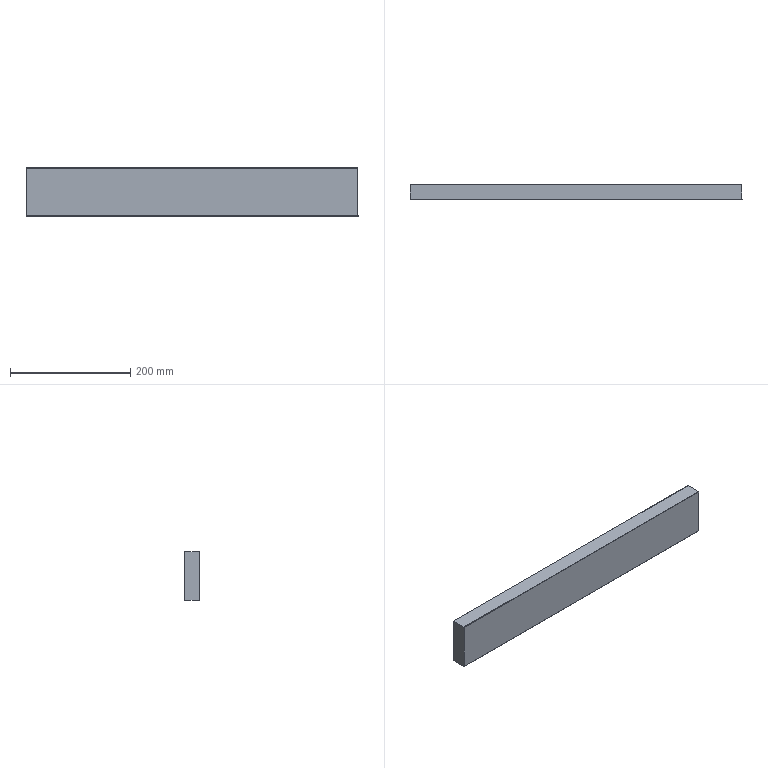Part | STEP file | DEWALT-DWE7492-B22 | 1 solid | 10 faces | box 552.2 x 25.6 x 80 mm | volume 1130787 mm3 | plane 6 | cylinder 4 | commonest cylinder face diameters 1 x4
STEP:
#1=CARTESIAN_POINT('',(0.,0.,0.));
#2=DIRECTION('',(0.,0.,1.));
#3=DIRECTION('',(1.,0.,0.));
#4=AXIS2_PLACEMENT_3D('',#1,#2,#3);
#5=CARTESIAN_POINT('',(-285.1,166.3,40.));
#6=VERTEX_POINT('',#5);
#7=CARTESIAN_POINT('',(-285.1,166.8,40.5));
#8=VERTEX_POINT('',#7);
#9=CARTESIAN_POINT('',(-285.1,166.3,40.5));
#10=DIRECTION('',(1.,0.,0.));
#11=DIRECTION('',(0.,0.,-1.));
#12=AXIS2_PLACEMENT_3D('',#9,#10,#11);
#13=CIRCLE('',#12,0.5);
#14=CARTESIAN_POINT('',(-285.1,166.3,40.5));
#15=DIRECTION('',(1.,0.,0.));
#16=DIRECTION('',(0.,0.,-1.));
#17=AXIS2_PLACEMENT_3D('',#14,#15,#16);
#18=CYLINDRICAL_SURFACE('',#17,0.5);
#19=CARTESIAN_POINT('',(0.,0.));
#20=DIRECTION('',(1.,0.));
#21=VECTOR('',#20,1.);
#22=LINE('',#19,#21);
#23=(GEOMETRIC_REPRESENTATION_CONTEXT(2)PARAMETRIC_REPRESENTATION_CONTEXT()REPRESENTATION_CONTEXT('',''));
#24=DEFINITIONAL_REPRESENTATION('',(#22),#23);
#25=PCURVE('',#18,#24);
#26=CARTESIAN_POINT('',(-285.1,141.19,39.99));
#27=DIRECTION('',(-1.,0.,0.));
#28=DIRECTION('',(0.,0.,1.));
#29=AXIS2_PLACEMENT_3D('',#26,#27,#28);
#30=PLANE('',#29);
#31=CARTESIAN_POINT('',(0.01,25.11));
#32=CARTESIAN_POINT('',(0.01,25.976));
#33=CARTESIAN_POINT('',(0.76,25.543));
#34=CARTESIAN_POINT('',(1.51,25.11));
#35=CARTESIAN_POINT('',(0.76,24.677));
#36=CARTESIAN_POINT('',(0.01,24.244));
#37=CARTESIAN_POINT('',(0.01,25.11));
#38=(BOUNDED_CURVE()B_SPLINE_CURVE(2,(#31,#32,#33,#34,#35,#36,#37),.UNSPECIFIED.,.T.,.F.)B_SPLINE_CURVE_WITH_KNOTS((1,2,2,2,2,1),(-2.094,0.,2.094,4.189,6.283,8.378),.UNSPECIFIED.)CURVE()GEOMETRIC_REPRESENTATION_ITEM()RATIONAL_B_SPLINE_CURVE((1.,0.5,1.,0.5,1.,0.5,1.))REPRESENTATION_ITEM(''));
#39=(GEOMETRIC_REPRESENTATION_CONTEXT(2)PARAMETRIC_REPRESENTATION_CONTEXT()REPRESENTATION_CONTEXT('',''));
#40=DEFINITIONAL_REPRESENTATION('',(#38),#39);
#41=PCURVE('',#30,#40);
#42=SURFACE_CURVE('',#13,(#25,#41),.PCURVE_S1.);
#43=EDGE_CURVE('',#6,#8,#42,.T.);
#44=ORIENTED_EDGE('',*,*,#43,.T.);
#45=CARTESIAN_POINT('',(267.1,166.8,40.5));
#46=VERTEX_POINT('',#45);
#47=CARTESIAN_POINT('',(-9.,166.8,40.5));
#48=DIRECTION('',(1.,0.,0.));
#49=VECTOR('',#48,1.);
#50=LINE('',#47,#49);
#51=CARTESIAN_POINT('',(1.571,276.1));
#52=DIRECTION('',(0.,1.));
#53=VECTOR('',#52,1.);
#54=LINE('',#51,#53);
#55=(GEOMETRIC_REPRESENTATION_CONTEXT(2)PARAMETRIC_REPRESENTATION_CONTEXT()REPRESENTATION_CONTEXT('',''));
#56=DEFINITIONAL_REPRESENTATION('',(#54),#55);
#57=PCURVE('',#18,#56);
#58=CARTESIAN_POINT('',(267.11,166.8,119.51));
#59=DIRECTION('',(0.,1.,0.));
#60=DIRECTION('',(0.,0.,-1.));
#61=AXIS2_PLACEMENT_3D('',#58,#59,#60);
#62=PLANE('',#61);
#63=CARTESIAN_POINT('',(79.01,276.11));
#64=DIRECTION('',(0.,-1.));
#65=VECTOR('',#64,1.);
#66=LINE('',#63,#65);
#67=(GEOMETRIC_REPRESENTATION_CONTEXT(2)PARAMETRIC_REPRESENTATION_CONTEXT()REPRESENTATION_CONTEXT('',''));
#68=DEFINITIONAL_REPRESENTATION('',(#66),#67);
#69=PCURVE('',#62,#68);
#70=SURFACE_CURVE('',#50,(#57,#69),.PCURVE_S1.);
#71=EDGE_CURVE('',#8,#46,#70,.T.);
#72=ORIENTED_EDGE('',*,*,#71,.T.);
#73=CARTESIAN_POINT('',(267.1,166.3,40.));
#74=VERTEX_POINT('',#73);
#75=CARTESIAN_POINT('',(267.1,166.3,40.5));
#76=DIRECTION('',(-1.,0.,0.));
#77=DIRECTION('',(0.,1.,0.));
#78=AXIS2_PLACEMENT_3D('',#75,#76,#77);
#79=CIRCLE('',#78,0.5);
#80=CARTESIAN_POINT('',(1.571,552.2));
#81=DIRECTION('',(-1.,0.));
#82=VECTOR('',#81,1.);
#83=LINE('',#80,#82);
#84=(GEOMETRIC_REPRESENTATION_CONTEXT(2)PARAMETRIC_REPRESENTATION_CONTEXT()REPRESENTATION_CONTEXT('',''));
#85=DEFINITIONAL_REPRESENTATION('',(#83),#84);
#86=PCURVE('',#18,#85);
#87=CARTESIAN_POINT('',(267.1,141.19,120.01));
#88=DIRECTION('',(1.,0.,0.));
#89=DIRECTION('',(0.,0.,-1.));
#90=AXIS2_PLACEMENT_3D('',#87,#88,#89);
#91=PLANE('',#90);
#92=CARTESIAN_POINT('',(79.51,25.61));
#93=CARTESIAN_POINT('',(80.376,25.61));
#94=CARTESIAN_POINT('',(79.943,24.86));
#95=CARTESIAN_POINT('',(79.51,24.11));
#96=CARTESIAN_POINT('',(79.077,24.86));
#97=CARTESIAN_POINT('',(78.644,25.61));
#98=CARTESIAN_POINT('',(79.51,25.61));
#99=(BOUNDED_CURVE()B_SPLINE_CURVE(2,(#92,#93,#94,#95,#96,#97,#98),.UNSPECIFIED.,.T.,.F.)B_SPLINE_CURVE_WITH_KNOTS((1,2,2,2,2,1),(-2.094,0.,2.094,4.189,6.283,8.378),.UNSPECIFIED.)CURVE()GEOMETRIC_REPRESENTATION_ITEM()RATIONAL_B_SPLINE_CURVE((1.,0.5,1.,0.5,1.,0.5,1.))REPRESENTATION_ITEM(''));
#100=(GEOMETRIC_REPRESENTATION_CONTEXT(2)PARAMETRIC_REPRESENTATION_CONTEXT()REPRESENTATION_CONTEXT('',''));
#101=DEFINITIONAL_REPRESENTATION('',(#99),#100);
#102=PCURVE('',#91,#101);
#103=SURFACE_CURVE('',#79,(#86,#102),.PCURVE_S1.);
#104=EDGE_CURVE('',#46,#74,#103,.T.);
#105=ORIENTED_EDGE('',*,*,#104,.T.);
#106=CARTESIAN_POINT('',(-9.,166.3,40.));
#107=DIRECTION('',(-1.,0.,0.));
#108=VECTOR('',#107,1.);
#109=LINE('',#106,#108);
#110=CARTESIAN_POINT('',(0.,276.1));
#111=DIRECTION('',(0.,-1.));
#112=VECTOR('',#111,1.);
#113=LINE('',#110,#112);
#114=(GEOMETRIC_REPRESENTATION_CONTEXT(2)PARAMETRIC_REPRESENTATION_CONTEXT()REPRESENTATION_CONTEXT('',''));
#115=DEFINITIONAL_REPRESENTATION('',(#113),#114);
#116=PCURVE('',#18,#115);
#117=CARTESIAN_POINT('',(267.11,166.31,40.));
#118=DIRECTION('',(0.,0.,-1.));
#119=DIRECTION('',(0.,-1.,0.));
#120=AXIS2_PLACEMENT_3D('',#117,#118,#119);
#121=PLANE('',#120);
#122=CARTESIAN_POINT('',(0.01,276.11));
#123=DIRECTION('',(0.,1.));
#124=VECTOR('',#123,1.);
#125=LINE('',#122,#124);
#126=(GEOMETRIC_REPRESENTATION_CONTEXT(2)PARAMETRIC_REPRESENTATION_CONTEXT()REPRESENTATION_CONTEXT('',''));
#127=DEFINITIONAL_REPRESENTATION('',(#125),#126);
#128=PCURVE('',#121,#127);
#129=SURFACE_CURVE('',#109,(#116,#128),.PCURVE_S1.);
#130=EDGE_CURVE('',#74,#6,#129,.T.);
#131=ORIENTED_EDGE('',*,*,#130,.T.);
#132=EDGE_LOOP('',(#44,#72,#105,#131));
#133=FACE_BOUND('',#132,.T.);
#134=ADVANCED_FACE('',(#133),#18,.T.);
#135=ORIENTED_EDGE('',*,*,#130,.F.);
#136=CARTESIAN_POINT('',(267.1,141.7,40.));
#137=VERTEX_POINT('',#136);
#138=CARTESIAN_POINT('',(267.1,154.,40.));
#139=DIRECTION('',(0.,-1.,0.));
#140=VECTOR('',#139,1.);
#141=LINE('',#138,#140);
#142=CARTESIAN_POINT('',(12.31,0.01));
#143=DIRECTION('',(1.,0.));
#144=VECTOR('',#143,1.);
#145=LINE('',#142,#144);
#146=(GEOMETRIC_REPRESENTATION_CONTEXT(2)PARAMETRIC_REPRESENTATION_CONTEXT()REPRESENTATION_CONTEXT('',''));
#147=DEFINITIONAL_REPRESENTATION('',(#145),#146);
#148=PCURVE('',#121,#147);
#149=CARTESIAN_POINT('',(80.01,12.81));
#150=DIRECTION('',(0.,-1.));
#151=VECTOR('',#150,1.);
#152=LINE('',#149,#151);
#153=(GEOMETRIC_REPRESENTATION_CONTEXT(2)PARAMETRIC_REPRESENTATION_CONTEXT()REPRESENTATION_CONTEXT('',''));
#154=DEFINITIONAL_REPRESENTATION('',(#152),#153);
#155=PCURVE('',#91,#154);
#156=SURFACE_CURVE('',#141,(#148,#155),.PCURVE_S1.);
#157=EDGE_CURVE('',#74,#137,#156,.T.);
#158=ORIENTED_EDGE('',*,*,#157,.T.);
#159=CARTESIAN_POINT('',(-285.1,141.7,40.));
#160=VERTEX_POINT('',#159);
#161=CARTESIAN_POINT('',(-9.,141.7,40.));
#162=DIRECTION('',(1.,0.,0.));
#163=VECTOR('',#162,1.);
#164=LINE('',#161,#163);
#165=CARTESIAN_POINT('',(24.61,276.11));
#166=DIRECTION('',(0.,-1.));
#167=VECTOR('',#166,1.);
#168=LINE('',#165,#167);
#169=(GEOMETRIC_REPRESENTATION_CONTEXT(2)PARAMETRIC_REPRESENTATION_CONTEXT()REPRESENTATION_CONTEXT('',''));
#170=DEFINITIONAL_REPRESENTATION('',(#168),#169);
#171=PCURVE('',#121,#170);
#172=CARTESIAN_POINT('',(-285.1,141.7,40.5));
#173=DIRECTION('',(1.,0.,0.));
#174=DIRECTION('',(0.,0.,-1.));
#175=AXIS2_PLACEMENT_3D('',#172,#173,#174);
#176=CYLINDRICAL_SURFACE('',#175,0.5);
#177=CARTESIAN_POINT('',(6.283,276.1));
#178=DIRECTION('',(0.,1.));
#179=VECTOR('',#178,1.);
#180=LINE('',#177,#179);
#181=(GEOMETRIC_REPRESENTATION_CONTEXT(2)PARAMETRIC_REPRESENTATION_CONTEXT()REPRESENTATION_CONTEXT('',''));
#182=DEFINITIONAL_REPRESENTATION('',(#180),#181);
#183=PCURVE('',#176,#182);
#184=SURFACE_CURVE('',#164,(#171,#183),.PCURVE_S1.);
#185=EDGE_CURVE('',#160,#137,#184,.T.);
#186=ORIENTED_EDGE('',*,*,#185,.F.);
#187=CARTESIAN_POINT('',(-285.1,154.,40.));
#188=DIRECTION('',(0.,1.,0.));
#189=VECTOR('',#188,1.);
#190=LINE('',#187,#189);
#191=CARTESIAN_POINT('',(12.31,552.21));
#192=DIRECTION('',(-1.,0.));
#193=VECTOR('',#192,1.);
#194=LINE('',#191,#193);
#195=(GEOMETRIC_REPRESENTATION_CONTEXT(2)PARAMETRIC_REPRESENTATION_CONTEXT()REPRESENTATION_CONTEXT('',''));
#196=DEFINITIONAL_REPRESENTATION('',(#194),#195);
#197=PCURVE('',#121,#196);
#198=CARTESIAN_POINT('',(0.01,12.81));
#199=DIRECTION('',(0.,1.));
#200=VECTOR('',#199,1.);
#201=LINE('',#198,#200);
#202=(GEOMETRIC_REPRESENTATION_CONTEXT(2)PARAMETRIC_REPRESENTATION_CONTEXT()REPRESENTATION_CONTEXT('',''));
#203=DEFINITIONAL_REPRESENTATION('',(#201),#202);
#204=PCURVE('',#30,#203);
#205=SURFACE_CURVE('',#190,(#197,#204),.PCURVE_S1.);
#206=EDGE_CURVE('',#160,#6,#205,.T.);
#207=ORIENTED_EDGE('',*,*,#206,.T.);
#208=EDGE_LOOP('',(#135,#158,#186,#207));
#209=FACE_BOUND('',#208,.T.);
#210=ADVANCED_FACE('',(#209),#121,.T.);
#211=ORIENTED_EDGE('',*,*,#104,.F.);
#212=CARTESIAN_POINT('',(267.1,166.8,119.5));
#213=VERTEX_POINT('',#212);
#214=CARTESIAN_POINT('',(267.1,166.8,80.));
#215=DIRECTION('',(0.,0.,-1.));
#216=VECTOR('',#215,1.);
#217=LINE('',#214,#216);
#218=CARTESIAN_POINT('',(40.01,25.61));
#219=DIRECTION('',(1.,0.));
#220=VECTOR('',#219,1.);
#221=LINE('',#218,#220);
#222=(GEOMETRIC_REPRESENTATION_CONTEXT(2)PARAMETRIC_REPRESENTATION_CONTEXT()REPRESENTATION_CONTEXT('',''));
#223=DEFINITIONAL_REPRESENTATION('',(#221),#222);
#224=PCURVE('',#91,#223);
#225=CARTESIAN_POINT('',(39.51,0.01));
#226=DIRECTION('',(1.,0.));
#227=VECTOR('',#226,1.);
#228=LINE('',#225,#227);
#229=(GEOMETRIC_REPRESENTATION_CONTEXT(2)PARAMETRIC_REPRESENTATION_CONTEXT()REPRESENTATION_CONTEXT('',''));
#230=DEFINITIONAL_REPRESENTATION('',(#228),#229);
#231=PCURVE('',#62,#230);
#232=SURFACE_CURVE('',#217,(#224,#231),.PCURVE_S1.);
#233=EDGE_CURVE('',#213,#46,#232,.T.);
#234=ORIENTED_EDGE('',*,*,#233,.F.);
#235=CARTESIAN_POINT('',(267.1,166.3,120.));
#236=VERTEX_POINT('',#235);
#237=CARTESIAN_POINT('',(267.1,166.3,119.5));
#238=DIRECTION('',(-1.,0.,0.));
#239=DIRECTION('',(0.,0.,1.));
#240=AXIS2_PLACEMENT_3D('',#237,#238,#239);
#241=CIRCLE('',#240,0.5);
#242=CARTESIAN_POINT('',(0.01,25.11));
#243=CARTESIAN_POINT('',(0.01,25.976));
#244=CARTESIAN_POINT('',(0.76,25.543));
#245=CARTESIAN_POINT('',(1.51,25.11));
#246=CARTESIAN_POINT('',(0.76,24.677));
#247=CARTESIAN_POINT('',(0.01,24.244));
#248=CARTESIAN_POINT('',(0.01,25.11));
#249=(BOUNDED_CURVE()B_SPLINE_CURVE(2,(#242,#243,#244,#245,#246,#247,#248),.UNSPECIFIED.,.T.,.F.)B_SPLINE_CURVE_WITH_KNOTS((1,2,2,2,2,1),(-2.094,0.,2.094,4.189,6.283,8.378),.UNSPECIFIED.)CURVE()GEOMETRIC_REPRESENTATION_ITEM()RATIONAL_B_SPLINE_CURVE((1.,0.5,1.,0.5,1.,0.5,1.))REPRESENTATION_ITEM(''));
#250=(GEOMETRIC_REPRESENTATION_CONTEXT(2)PARAMETRIC_REPRESENTATION_CONTEXT()REPRESENTATION_CONTEXT('',''));
#251=DEFINITIONAL_REPRESENTATION('',(#249),#250);
#252=PCURVE('',#91,#251);
#253=CARTESIAN_POINT('',(-285.1,166.3,119.5));
#254=DIRECTION('',(1.,0.,0.));
#255=DIRECTION('',(0.,0.,-1.));
#256=AXIS2_PLACEMENT_3D('',#253,#254,#255);
#257=CYLINDRICAL_SURFACE('',#256,0.5);
#258=CARTESIAN_POINT('',(3.142,552.2));
#259=DIRECTION('',(-1.,0.));
#260=VECTOR('',#259,1.);
#261=LINE('',#258,#260);
#262=(GEOMETRIC_REPRESENTATION_CONTEXT(2)PARAMETRIC_REPRESENTATION_CONTEXT()REPRESENTATION_CONTEXT('',''));
#263=DEFINITIONAL_REPRESENTATION('',(#261),#262);
#264=PCURVE('',#257,#263);
#265=SURFACE_CURVE('',#241,(#252,#264),.PCURVE_S1.);
#266=EDGE_CURVE('',#236,#213,#265,.T.);
#267=ORIENTED_EDGE('',*,*,#266,.F.);
#268=CARTESIAN_POINT('',(267.1,141.7,120.));
#269=VERTEX_POINT('',#268);
#270=CARTESIAN_POINT('',(267.1,154.,120.));
#271=DIRECTION('',(0.,1.,0.));
#272=VECTOR('',#271,1.);
#273=LINE('',#270,#272);
#274=CARTESIAN_POINT('',(0.01,12.81));
#275=DIRECTION('',(0.,1.));
#276=VECTOR('',#275,1.);
#277=LINE('',#274,#276);
#278=(GEOMETRIC_REPRESENTATION_CONTEXT(2)PARAMETRIC_REPRESENTATION_CONTEXT()REPRESENTATION_CONTEXT('',''));
#279=DEFINITIONAL_REPRESENTATION('',(#277),#278);
#280=PCURVE('',#91,#279);
#281=CARTESIAN_POINT('',(267.11,141.69,120.));
#282=DIRECTION('',(0.,0.,1.));
#283=DIRECTION('',(0.,1.,0.));
#284=AXIS2_PLACEMENT_3D('',#281,#282,#283);
#285=PLANE('',#284);
#286=CARTESIAN_POINT('',(12.31,0.01));
#287=DIRECTION('',(1.,0.));
#288=VECTOR('',#287,1.);
#289=LINE('',#286,#288);
#290=(GEOMETRIC_REPRESENTATION_CONTEXT(2)PARAMETRIC_REPRESENTATION_CONTEXT()REPRESENTATION_CONTEXT('',''));
#291=DEFINITIONAL_REPRESENTATION('',(#289),#290);
#292=PCURVE('',#285,#291);
#293=SURFACE_CURVE('',#273,(#280,#292),.PCURVE_S1.);
#294=EDGE_CURVE('',#269,#236,#293,.T.);
#295=ORIENTED_EDGE('',*,*,#294,.F.);
#296=CARTESIAN_POINT('',(267.1,141.2,119.5));
#297=VERTEX_POINT('',#296);
#298=CARTESIAN_POINT('',(267.1,141.7,119.5));
#299=DIRECTION('',(-1.,0.,0.));
#300=DIRECTION('',(0.,-1.,0.));
#301=AXIS2_PLACEMENT_3D('',#298,#299,#300);
#302=CIRCLE('',#301,0.5);
#303=CARTESIAN_POINT('',(0.51,0.01));
#304=CARTESIAN_POINT('',(-0.356,0.01));
#305=CARTESIAN_POINT('',(0.07699,0.76));
#306=CARTESIAN_POINT('',(0.51,1.51));
#307=CARTESIAN_POINT('',(0.943,0.76));
#308=CARTESIAN_POINT('',(1.376,0.01));
#309=CARTESIAN_POINT('',(0.51,0.01));
#310=(BOUNDED_CURVE()B_SPLINE_CURVE(2,(#303,#304,#305,#306,#307,#308,#309),.UNSPECIFIED.,.T.,.F.)B_SPLINE_CURVE_WITH_KNOTS((1,2,2,2,2,1),(-2.094,0.,2.094,4.189,6.283,8.378),.UNSPECIFIED.)CURVE()GEOMETRIC_REPRESENTATION_ITEM()RATIONAL_B_SPLINE_CURVE((1.,0.5,1.,0.5,1.,0.5,1.))REPRESENTATION_ITEM(''));
#311=(GEOMETRIC_REPRESENTATION_CONTEXT(2)PARAMETRIC_REPRESENTATION_CONTEXT()REPRESENTATION_CONTEXT('',''));
#312=DEFINITIONAL_REPRESENTATION('',(#310),#311);
#313=PCURVE('',#91,#312);
#314=CARTESIAN_POINT('',(-285.1,141.7,119.5));
#315=DIRECTION('',(1.,0.,0.));
#316=DIRECTION('',(0.,0.,-1.));
#317=AXIS2_PLACEMENT_3D('',#314,#315,#316);
#318=CYLINDRICAL_SURFACE('',#317,0.5);
#319=CARTESIAN_POINT('',(4.712,552.2));
#320=DIRECTION('',(-1.,0.));
#321=VECTOR('',#320,1.);
#322=LINE('',#319,#321);
#323=(GEOMETRIC_REPRESENTATION_CONTEXT(2)PARAMETRIC_REPRESENTATION_CONTEXT()REPRESENTATION_CONTEXT('',''));
#324=DEFINITIONAL_REPRESENTATION('',(#322),#323);
#325=PCURVE('',#318,#324);
#326=SURFACE_CURVE('',#302,(#313,#325),.PCURVE_S1.);
#327=EDGE_CURVE('',#297,#269,#326,.T.);
#328=ORIENTED_EDGE('',*,*,#327,.F.);
#329=CARTESIAN_POINT('',(267.1,141.2,40.5));
#330=VERTEX_POINT('',#329);
#331=CARTESIAN_POINT('',(267.1,141.2,80.));
#332=DIRECTION('',(0.,0.,1.));
#333=VECTOR('',#332,1.);
#334=LINE('',#331,#333);
#335=CARTESIAN_POINT('',(40.01,0.01));
#336=DIRECTION('',(-1.,0.));
#337=VECTOR('',#336,1.);
#338=LINE('',#335,#337);
#339=(GEOMETRIC_REPRESENTATION_CONTEXT(2)PARAMETRIC_REPRESENTATION_CONTEXT()REPRESENTATION_CONTEXT('',''));
#340=DEFINITIONAL_REPRESENTATION('',(#338),#339);
#341=PCURVE('',#91,#340);
#342=CARTESIAN_POINT('',(267.11,141.2,40.49));
#343=DIRECTION('',(0.,-1.,0.));
#344=DIRECTION('',(0.,0.,1.));
#345=AXIS2_PLACEMENT_3D('',#342,#343,#344);
#346=PLANE('',#345);
#347=CARTESIAN_POINT('',(39.51,0.01));
#348=DIRECTION('',(1.,0.));
#349=VECTOR('',#348,1.);
#350=LINE('',#347,#349);
#351=(GEOMETRIC_REPRESENTATION_CONTEXT(2)PARAMETRIC_REPRESENTATION_CONTEXT()REPRESENTATION_CONTEXT('',''));
#352=DEFINITIONAL_REPRESENTATION('',(#350),#351);
#353=PCURVE('',#346,#352);
#354=SURFACE_CURVE('',#334,(#341,#353),.PCURVE_S1.);
#355=EDGE_CURVE('',#330,#297,#354,.T.);
#356=ORIENTED_EDGE('',*,*,#355,.F.);
#357=CARTESIAN_POINT('',(267.1,141.7,40.5));
#358=DIRECTION('',(-1.,0.,0.));
#359=DIRECTION('',(0.,0.,-1.));
#360=AXIS2_PLACEMENT_3D('',#357,#358,#359);
#361=CIRCLE('',#360,0.5);
#362=CARTESIAN_POINT('',(80.01,0.51));
#363=CARTESIAN_POINT('',(80.01,-0.356));
#364=CARTESIAN_POINT('',(79.26,0.07699));
#365=CARTESIAN_POINT('',(78.51,0.51));
#366=CARTESIAN_POINT('',(79.26,0.943));
#367=CARTESIAN_POINT('',(80.01,1.376));
#368=CARTESIAN_POINT('',(80.01,0.51));
#369=(BOUNDED_CURVE()B_SPLINE_CURVE(2,(#362,#363,#364,#365,#366,#367,#368),.UNSPECIFIED.,.T.,.F.)B_SPLINE_CURVE_WITH_KNOTS((1,2,2,2,2,1),(-2.094,0.,2.094,4.189,6.283,8.378),.UNSPECIFIED.)CURVE()GEOMETRIC_REPRESENTATION_ITEM()RATIONAL_B_SPLINE_CURVE((1.,0.5,1.,0.5,1.,0.5,1.))REPRESENTATION_ITEM(''));
#370=(GEOMETRIC_REPRESENTATION_CONTEXT(2)PARAMETRIC_REPRESENTATION_CONTEXT()REPRESENTATION_CONTEXT('',''));
#371=DEFINITIONAL_REPRESENTATION('',(#369),#370);
#372=PCURVE('',#91,#371);
#373=CARTESIAN_POINT('',(6.283,552.2));
#374=DIRECTION('',(-1.,0.));
#375=VECTOR('',#374,1.);
#376=LINE('',#373,#375);
#377=(GEOMETRIC_REPRESENTATION_CONTEXT(2)PARAMETRIC_REPRESENTATION_CONTEXT()REPRESENTATION_CONTEXT('',''));
#378=DEFINITIONAL_REPRESENTATION('',(#376),#377);
#379=PCURVE('',#176,#378);
#380=SURFACE_CURVE('',#361,(#372,#379),.PCURVE_S1.);
#381=EDGE_CURVE('',#137,#330,#380,.T.);
#382=ORIENTED_EDGE('',*,*,#381,.F.);
#383=ORIENTED_EDGE('',*,*,#157,.F.);
#384=EDGE_LOOP('',(#211,#234,#267,#295,#328,#356,#382,#383));
#385=FACE_BOUND('',#384,.T.);
#386=ADVANCED_FACE('',(#385),#91,.T.);
#387=CARTESIAN_POINT('',(-285.1,166.8,119.5));
#388=VERTEX_POINT('',#387);
#389=CARTESIAN_POINT('',(-285.1,166.3,120.));
#390=VERTEX_POINT('',#389);
#391=CARTESIAN_POINT('',(-285.1,166.3,119.5));
#392=DIRECTION('',(1.,0.,0.));
#393=DIRECTION('',(0.,1.,0.));
#394=AXIS2_PLACEMENT_3D('',#391,#392,#393);
#395=CIRCLE('',#394,0.5);
#396=CARTESIAN_POINT('',(1.571,0.));
#397=DIRECTION('',(1.,0.));
#398=VECTOR('',#397,1.);
#399=LINE('',#396,#398);
#400=(GEOMETRIC_REPRESENTATION_CONTEXT(2)PARAMETRIC_REPRESENTATION_CONTEXT()REPRESENTATION_CONTEXT('',''));
#401=DEFINITIONAL_REPRESENTATION('',(#399),#400);
#402=PCURVE('',#257,#401);
#403=CARTESIAN_POINT('',(79.51,25.61));
#404=CARTESIAN_POINT('',(80.376,25.61));
#405=CARTESIAN_POINT('',(79.943,24.86));
#406=CARTESIAN_POINT('',(79.51,24.11));
#407=CARTESIAN_POINT('',(79.077,24.86));
#408=CARTESIAN_POINT('',(78.644,25.61));
#409=CARTESIAN_POINT('',(79.51,25.61));
#410=(BOUNDED_CURVE()B_SPLINE_CURVE(2,(#403,#404,#405,#406,#407,#408,#409),.UNSPECIFIED.,.T.,.F.)B_SPLINE_CURVE_WITH_KNOTS((1,2,2,2,2,1),(-2.094,0.,2.094,4.189,6.283,8.378),.UNSPECIFIED.)CURVE()GEOMETRIC_REPRESENTATION_ITEM()RATIONAL_B_SPLINE_CURVE((1.,0.5,1.,0.5,1.,0.5,1.))REPRESENTATION_ITEM(''));
#411=(GEOMETRIC_REPRESENTATION_CONTEXT(2)PARAMETRIC_REPRESENTATION_CONTEXT()REPRESENTATION_CONTEXT('',''));
#412=DEFINITIONAL_REPRESENTATION('',(#410),#411);
#413=PCURVE('',#30,#412);
#414=SURFACE_CURVE('',#395,(#402,#413),.PCURVE_S1.);
#415=EDGE_CURVE('',#388,#390,#414,.T.);
#416=ORIENTED_EDGE('',*,*,#415,.T.);
#417=CARTESIAN_POINT('',(-9.,166.3,120.));
#418=DIRECTION('',(1.,0.,0.));
#419=VECTOR('',#418,1.);
#420=LINE('',#417,#419);
#421=CARTESIAN_POINT('',(3.142,276.1));
#422=DIRECTION('',(0.,1.));
#423=VECTOR('',#422,1.);
#424=LINE('',#421,#423);
#425=(GEOMETRIC_REPRESENTATION_CONTEXT(2)PARAMETRIC_REPRESENTATION_CONTEXT()REPRESENTATION_CONTEXT('',''));
#426=DEFINITIONAL_REPRESENTATION('',(#424),#425);
#427=PCURVE('',#257,#426);
#428=CARTESIAN_POINT('',(24.61,276.11));
#429=DIRECTION('',(0.,-1.));
#430=VECTOR('',#429,1.);
#431=LINE('',#428,#430);
#432=(GEOMETRIC_REPRESENTATION_CONTEXT(2)PARAMETRIC_REPRESENTATION_CONTEXT()REPRESENTATION_CONTEXT('',''));
#433=DEFINITIONAL_REPRESENTATION('',(#431),#432);
#434=PCURVE('',#285,#433);
#435=SURFACE_CURVE('',#420,(#427,#434),.PCURVE_S1.);
#436=EDGE_CURVE('',#390,#236,#435,.T.);
#437=ORIENTED_EDGE('',*,*,#436,.T.);
#438=ORIENTED_EDGE('',*,*,#266,.T.);
#439=CARTESIAN_POINT('',(-9.,166.8,119.5));
#440=DIRECTION('',(-1.,0.,0.));
#441=VECTOR('',#440,1.);
#442=LINE('',#439,#441);
#443=CARTESIAN_POINT('',(1.571,276.1));
#444=DIRECTION('',(0.,-1.));
#445=VECTOR('',#444,1.);
#446=LINE('',#443,#445);
#447=(GEOMETRIC_REPRESENTATION_CONTEXT(2)PARAMETRIC_REPRESENTATION_CONTEXT()REPRESENTATION_CONTEXT('',''));
#448=DEFINITIONAL_REPRESENTATION('',(#446),#447);
#449=PCURVE('',#257,#448);
#450=CARTESIAN_POINT('',(0.01,276.11));
#451=DIRECTION('',(0.,1.));
#452=VECTOR('',#451,1.);
#453=LINE('',#450,#452);
#454=(GEOMETRIC_REPRESENTATION_CONTEXT(2)PARAMETRIC_REPRESENTATION_CONTEXT()REPRESENTATION_CONTEXT('',''));
#455=DEFINITIONAL_REPRESENTATION('',(#453),#454);
#456=PCURVE('',#62,#455);
#457=SURFACE_CURVE('',#442,(#449,#456),.PCURVE_S1.);
#458=EDGE_CURVE('',#213,#388,#457,.T.);
#459=ORIENTED_EDGE('',*,*,#458,.T.);
#460=EDGE_LOOP('',(#416,#437,#438,#459));
#461=FACE_BOUND('',#460,.T.);
#462=ADVANCED_FACE('',(#461),#257,.T.);
#463=ORIENTED_EDGE('',*,*,#436,.F.);
#464=CARTESIAN_POINT('',(-285.1,141.7,120.));
#465=VERTEX_POINT('',#464);
#466=CARTESIAN_POINT('',(-285.1,154.,120.));
#467=DIRECTION('',(0.,-1.,0.));
#468=VECTOR('',#467,1.);
#469=LINE('',#466,#468);
#470=CARTESIAN_POINT('',(12.31,552.21));
#471=DIRECTION('',(-1.,0.));
#472=VECTOR('',#471,1.);
#473=LINE('',#470,#472);
#474=(GEOMETRIC_REPRESENTATION_CONTEXT(2)PARAMETRIC_REPRESENTATION_CONTEXT()REPRESENTATION_CONTEXT('',''));
#475=DEFINITIONAL_REPRESENTATION('',(#473),#474);
#476=PCURVE('',#285,#475);
#477=CARTESIAN_POINT('',(80.01,12.81));
#478=DIRECTION('',(0.,-1.));
#479=VECTOR('',#478,1.);
#480=LINE('',#477,#479);
#481=(GEOMETRIC_REPRESENTATION_CONTEXT(2)PARAMETRIC_REPRESENTATION_CONTEXT()REPRESENTATION_CONTEXT('',''));
#482=DEFINITIONAL_REPRESENTATION('',(#480),#481);
#483=PCURVE('',#30,#482);
#484=SURFACE_CURVE('',#469,(#476,#483),.PCURVE_S1.);
#485=EDGE_CURVE('',#390,#465,#484,.T.);
#486=ORIENTED_EDGE('',*,*,#485,.T.);
#487=CARTESIAN_POINT('',(-9.,141.7,120.));
#488=DIRECTION('',(-1.,0.,0.));
#489=VECTOR('',#488,1.);
#490=LINE('',#487,#489);
#491=CARTESIAN_POINT('',(0.01,276.11));
#492=DIRECTION('',(0.,1.));
#493=VECTOR('',#492,1.);
#494=LINE('',#491,#493);
#495=(GEOMETRIC_REPRESENTATION_CONTEXT(2)PARAMETRIC_REPRESENTATION_CONTEXT()REPRESENTATION_CONTEXT('',''));
#496=DEFINITIONAL_REPRESENTATION('',(#494),#495);
#497=PCURVE('',#285,#496);
#498=CARTESIAN_POINT('',(3.142,276.1));
#499=DIRECTION('',(0.,-1.));
#500=VECTOR('',#499,1.);
#501=LINE('',#498,#500);
#502=(GEOMETRIC_REPRESENTATION_CONTEXT(2)PARAMETRIC_REPRESENTATION_CONTEXT()REPRESENTATION_CONTEXT('',''));
#503=DEFINITIONAL_REPRESENTATION('',(#501),#502);
#504=PCURVE('',#318,#503);
#505=SURFACE_CURVE('',#490,(#497,#504),.PCURVE_S1.);
#506=EDGE_CURVE('',#269,#465,#505,.T.);
#507=ORIENTED_EDGE('',*,*,#506,.F.);
#508=ORIENTED_EDGE('',*,*,#294,.T.);
#509=EDGE_LOOP('',(#463,#486,#507,#508));
#510=FACE_BOUND('',#509,.T.);
#511=ADVANCED_FACE('',(#510),#285,.T.);
#512=ORIENTED_EDGE('',*,*,#43,.F.);
#513=ORIENTED_EDGE('',*,*,#206,.F.);
#514=CARTESIAN_POINT('',(-285.1,141.2,40.5));
#515=VERTEX_POINT('',#514);
#516=CARTESIAN_POINT('',(-285.1,141.7,40.5));
#517=DIRECTION('',(1.,0.,0.));
#518=DIRECTION('',(0.,-1.,0.));
#519=AXIS2_PLACEMENT_3D('',#516,#517,#518);
#520=CIRCLE('',#519,0.5);
#521=CARTESIAN_POINT('',(0.51,0.01));
#522=CARTESIAN_POINT('',(-0.356,0.01));
#523=CARTESIAN_POINT('',(0.07699,0.76));
#524=CARTESIAN_POINT('',(0.51,1.51));
#525=CARTESIAN_POINT('',(0.943,0.76));
#526=CARTESIAN_POINT('',(1.376,0.01));
#527=CARTESIAN_POINT('',(0.51,0.01));
#528=(BOUNDED_CURVE()B_SPLINE_CURVE(2,(#521,#522,#523,#524,#525,#526,#527),.UNSPECIFIED.,.T.,.F.)B_SPLINE_CURVE_WITH_KNOTS((1,2,2,2,2,1),(-2.094,0.,2.094,4.189,6.283,8.378),.UNSPECIFIED.)CURVE()GEOMETRIC_REPRESENTATION_ITEM()RATIONAL_B_SPLINE_CURVE((1.,0.5,1.,0.5,1.,0.5,1.))REPRESENTATION_ITEM(''));
#529=(GEOMETRIC_REPRESENTATION_CONTEXT(2)PARAMETRIC_REPRESENTATION_CONTEXT()REPRESENTATION_CONTEXT('',''));
#530=DEFINITIONAL_REPRESENTATION('',(#528),#529);
#531=PCURVE('',#30,#530);
#532=CARTESIAN_POINT('',(4.712,0.));
#533=DIRECTION('',(1.,0.));
#534=VECTOR('',#533,1.);
#535=LINE('',#532,#534);
#536=(GEOMETRIC_REPRESENTATION_CONTEXT(2)PARAMETRIC_REPRESENTATION_CONTEXT()REPRESENTATION_CONTEXT('',''));
#537=DEFINITIONAL_REPRESENTATION('',(#535),#536);
#538=PCURVE('',#176,#537);
#539=SURFACE_CURVE('',#520,(#531,#538),.PCURVE_S1.);
#540=EDGE_CURVE('',#515,#160,#539,.T.);
#541=ORIENTED_EDGE('',*,*,#540,.F.);
#542=CARTESIAN_POINT('',(-285.1,141.2,119.5));
#543=VERTEX_POINT('',#542);
#544=CARTESIAN_POINT('',(-285.1,141.2,80.));
#545=DIRECTION('',(0.,0.,-1.));
#546=VECTOR('',#545,1.);
#547=LINE('',#544,#546);
#548=CARTESIAN_POINT('',(40.01,0.01));
#549=DIRECTION('',(-1.,0.));
#550=VECTOR('',#549,1.);
#551=LINE('',#548,#550);
#552=(GEOMETRIC_REPRESENTATION_CONTEXT(2)PARAMETRIC_REPRESENTATION_CONTEXT()REPRESENTATION_CONTEXT('',''));
#553=DEFINITIONAL_REPRESENTATION('',(#551),#552);
#554=PCURVE('',#30,#553);
#555=CARTESIAN_POINT('',(39.51,552.21));
#556=DIRECTION('',(-1.,0.));
#557=VECTOR('',#556,1.);
#558=LINE('',#555,#557);
#559=(GEOMETRIC_REPRESENTATION_CONTEXT(2)PARAMETRIC_REPRESENTATION_CONTEXT()REPRESENTATION_CONTEXT('',''));
#560=DEFINITIONAL_REPRESENTATION('',(#558),#559);
#561=PCURVE('',#346,#560);
#562=SURFACE_CURVE('',#547,(#554,#561),.PCURVE_S1.);
#563=EDGE_CURVE('',#543,#515,#562,.T.);
#564=ORIENTED_EDGE('',*,*,#563,.F.);
#565=CARTESIAN_POINT('',(-285.1,141.7,119.5));
#566=DIRECTION('',(1.,0.,0.));
#567=DIRECTION('',(0.,0.,1.));
#568=AXIS2_PLACEMENT_3D('',#565,#566,#567);
#569=CIRCLE('',#568,0.5);
#570=CARTESIAN_POINT('',(80.01,0.51));
#571=CARTESIAN_POINT('',(80.01,-0.356));
#572=CARTESIAN_POINT('',(79.26,0.07699));
#573=CARTESIAN_POINT('',(78.51,0.51));
#574=CARTESIAN_POINT('',(79.26,0.943));
#575=CARTESIAN_POINT('',(80.01,1.376));
#576=CARTESIAN_POINT('',(80.01,0.51));
#577=(BOUNDED_CURVE()B_SPLINE_CURVE(2,(#570,#571,#572,#573,#574,#575,#576),.UNSPECIFIED.,.T.,.F.)B_SPLINE_CURVE_WITH_KNOTS((1,2,2,2,2,1),(-2.094,0.,2.094,4.189,6.283,8.378),.UNSPECIFIED.)CURVE()GEOMETRIC_REPRESENTATION_ITEM()RATIONAL_B_SPLINE_CURVE((1.,0.5,1.,0.5,1.,0.5,1.))REPRESENTATION_ITEM(''));
#578=(GEOMETRIC_REPRESENTATION_CONTEXT(2)PARAMETRIC_REPRESENTATION_CONTEXT()REPRESENTATION_CONTEXT('',''));
#579=DEFINITIONAL_REPRESENTATION('',(#577),#578);
#580=PCURVE('',#30,#579);
#581=CARTESIAN_POINT('',(3.142,0.));
#582=DIRECTION('',(1.,0.));
#583=VECTOR('',#582,1.);
#584=LINE('',#581,#583);
#585=(GEOMETRIC_REPRESENTATION_CONTEXT(2)PARAMETRIC_REPRESENTATION_CONTEXT()REPRESENTATION_CONTEXT('',''));
#586=DEFINITIONAL_REPRESENTATION('',(#584),#585);
#587=PCURVE('',#318,#586);
#588=SURFACE_CURVE('',#569,(#580,#587),.PCURVE_S1.);
#589=EDGE_CURVE('',#465,#543,#588,.T.);
#590=ORIENTED_EDGE('',*,*,#589,.F.);
#591=ORIENTED_EDGE('',*,*,#485,.F.);
#592=ORIENTED_EDGE('',*,*,#415,.F.);
#593=CARTESIAN_POINT('',(-285.1,166.8,80.));
#594=DIRECTION('',(0.,0.,1.));
#595=VECTOR('',#594,1.);
#596=LINE('',#593,#595);
#597=CARTESIAN_POINT('',(40.01,25.61));
#598=DIRECTION('',(1.,0.));
#599=VECTOR('',#598,1.);
#600=LINE('',#597,#599);
#601=(GEOMETRIC_REPRESENTATION_CONTEXT(2)PARAMETRIC_REPRESENTATION_CONTEXT()REPRESENTATION_CONTEXT('',''));
#602=DEFINITIONAL_REPRESENTATION('',(#600),#601);
#603=PCURVE('',#30,#602);
#604=CARTESIAN_POINT('',(39.51,552.21));
#605=DIRECTION('',(-1.,0.));
#606=VECTOR('',#605,1.);
#607=LINE('',#604,#606);
#608=(GEOMETRIC_REPRESENTATION_CONTEXT(2)PARAMETRIC_REPRESENTATION_CONTEXT()REPRESENTATION_CONTEXT('',''));
#609=DEFINITIONAL_REPRESENTATION('',(#607),#608);
#610=PCURVE('',#62,#609);
#611=SURFACE_CURVE('',#596,(#603,#610),.PCURVE_S1.);
#612=EDGE_CURVE('',#8,#388,#611,.T.);
#613=ORIENTED_EDGE('',*,*,#612,.F.);
#614=EDGE_LOOP('',(#512,#513,#541,#564,#590,#591,#592,#613));
#615=FACE_BOUND('',#614,.T.);
#616=ADVANCED_FACE('',(#615),#30,.T.);
#617=ORIENTED_EDGE('',*,*,#589,.T.);
#618=CARTESIAN_POINT('',(-9.,141.2,119.5));
#619=DIRECTION('',(1.,0.,0.));
#620=VECTOR('',#619,1.);
#621=LINE('',#618,#620);
#622=CARTESIAN_POINT('',(4.712,276.1));
#623=DIRECTION('',(0.,1.));
#624=VECTOR('',#623,1.);
#625=LINE('',#622,#624);
#626=(GEOMETRIC_REPRESENTATION_CONTEXT(2)PARAMETRIC_REPRESENTATION_CONTEXT()REPRESENTATION_CONTEXT('',''));
#627=DEFINITIONAL_REPRESENTATION('',(#625),#626);
#628=PCURVE('',#318,#627);
#629=CARTESIAN_POINT('',(79.01,276.11));
#630=DIRECTION('',(0.,-1.));
#631=VECTOR('',#630,1.);
#632=LINE('',#629,#631);
#633=(GEOMETRIC_REPRESENTATION_CONTEXT(2)PARAMETRIC_REPRESENTATION_CONTEXT()REPRESENTATION_CONTEXT('',''));
#634=DEFINITIONAL_REPRESENTATION('',(#632),#633);
#635=PCURVE('',#346,#634);
#636=SURFACE_CURVE('',#621,(#628,#635),.PCURVE_S1.);
#637=EDGE_CURVE('',#543,#297,#636,.T.);
#638=ORIENTED_EDGE('',*,*,#637,.T.);
#639=ORIENTED_EDGE('',*,*,#327,.T.);
#640=ORIENTED_EDGE('',*,*,#506,.T.);
#641=EDGE_LOOP('',(#617,#638,#639,#640));
#642=FACE_BOUND('',#641,.T.);
#643=ADVANCED_FACE('',(#642),#318,.T.);
#644=ORIENTED_EDGE('',*,*,#637,.F.);
#645=ORIENTED_EDGE('',*,*,#563,.T.);
#646=CARTESIAN_POINT('',(-9.,141.2,40.5));
#647=DIRECTION('',(-1.,0.,0.));
#648=VECTOR('',#647,1.);
#649=LINE('',#646,#648);
#650=CARTESIAN_POINT('',(0.01,276.11));
#651=DIRECTION('',(0.,1.));
#652=VECTOR('',#651,1.);
#653=LINE('',#650,#652);
#654=(GEOMETRIC_REPRESENTATION_CONTEXT(2)PARAMETRIC_REPRESENTATION_CONTEXT()REPRESENTATION_CONTEXT('',''));
#655=DEFINITIONAL_REPRESENTATION('',(#653),#654);
#656=PCURVE('',#346,#655);
#657=CARTESIAN_POINT('',(4.712,276.1));
#658=DIRECTION('',(0.,-1.));
#659=VECTOR('',#658,1.);
#660=LINE('',#657,#659);
#661=(GEOMETRIC_REPRESENTATION_CONTEXT(2)PARAMETRIC_REPRESENTATION_CONTEXT()REPRESENTATION_CONTEXT('',''));
#662=DEFINITIONAL_REPRESENTATION('',(#660),#661);
#663=PCURVE('',#176,#662);
#664=SURFACE_CURVE('',#649,(#656,#663),.PCURVE_S1.);
#665=EDGE_CURVE('',#330,#515,#664,.T.);
#666=ORIENTED_EDGE('',*,*,#665,.F.);
#667=ORIENTED_EDGE('',*,*,#355,.T.);
#668=EDGE_LOOP('',(#644,#645,#666,#667));
#669=FACE_BOUND('',#668,.T.);
#670=ADVANCED_FACE('',(#669),#346,.T.);
#671=ORIENTED_EDGE('',*,*,#540,.T.);
#672=ORIENTED_EDGE('',*,*,#185,.T.);
#673=ORIENTED_EDGE('',*,*,#381,.T.);
#674=ORIENTED_EDGE('',*,*,#665,.T.);
#675=EDGE_LOOP('',(#671,#672,#673,#674));
#676=FACE_BOUND('',#675,.T.);
#677=ADVANCED_FACE('',(#676),#176,.T.);
#678=ORIENTED_EDGE('',*,*,#71,.F.);
#679=ORIENTED_EDGE('',*,*,#612,.T.);
#680=ORIENTED_EDGE('',*,*,#458,.F.);
#681=ORIENTED_EDGE('',*,*,#233,.T.);
#682=EDGE_LOOP('',(#678,#679,#680,#681));
#683=FACE_BOUND('',#682,.T.);
#684=ADVANCED_FACE('',(#683),#62,.T.);
#685=CLOSED_SHELL('',(#134,#210,#386,#462,#511,#616,#643,#670,#677,#684));
#686=MANIFOLD_SOLID_BREP('',#685);
#687=(LENGTH_UNIT()NAMED_UNIT(*)SI_UNIT(.MILLI.,.METRE.));
#688=UNCERTAINTY_MEASURE_WITH_UNIT(LENGTH_MEASURE(0.0000001),#687,'','');
#689=(NAMED_UNIT(*)PLANE_ANGLE_UNIT()SI_UNIT($,.RADIAN.));
#690=(NAMED_UNIT(*)SI_UNIT($,.STERADIAN.)SOLID_ANGLE_UNIT());
#691=(GEOMETRIC_REPRESENTATION_CONTEXT(3)GLOBAL_UNCERTAINTY_ASSIGNED_CONTEXT((#688))GLOBAL_UNIT_ASSIGNED_CONTEXT((#687,#689,#690))REPRESENTATION_CONTEXT('',''));
#692=ADVANCED_BREP_SHAPE_REPRESENTATION('',(#4,#686),#691);